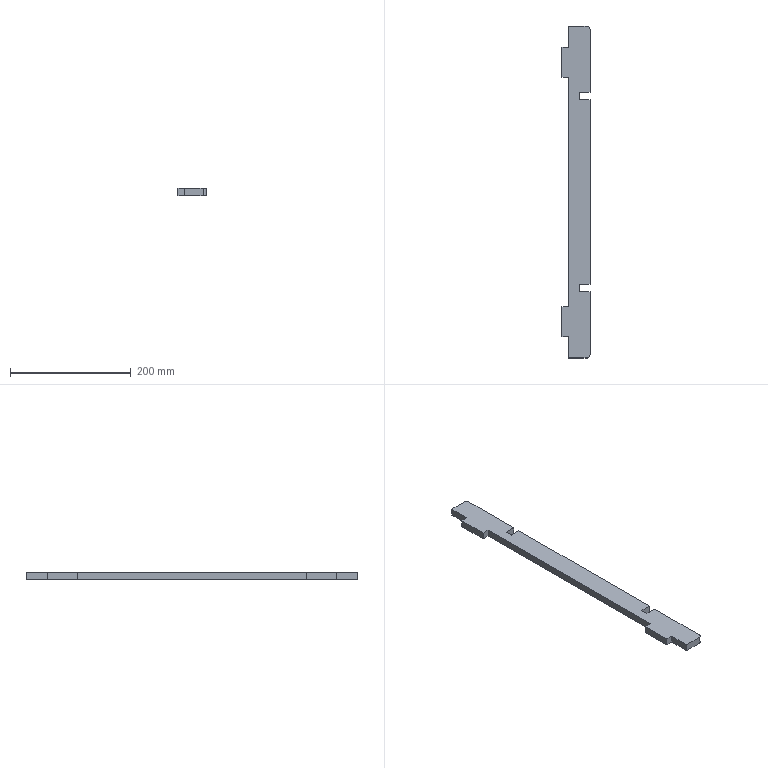Part | SolidWorks | features FlatPattern 1, SMBaseFlange 1, SheetMetal 1 | 1 solid | 24 faces | box 46.5 x 550 x 12 mm | volume 239574 mm3 | plane 22 | cylinder 2 | commonest cylinder face diameters 10 x2
STEP:
#1=CARTESIAN_POINT('',(-232.937,-290.509,0.));
#2=VERTEX_POINT('',#1);
#3=CARTESIAN_POINT('',(-232.937,-325.509,0.));
#4=VERTEX_POINT('',#3);
#5=CARTESIAN_POINT('',(-232.937,-325.509,0.));
#6=DIRECTION('',(0.,-1.,0.));
#7=VECTOR('',#6,1000.);
#8=LINE('',#5,#7);
#9=EDGE_CURVE('',#2,#4,#8,.T.);
#10=ORIENTED_EDGE('',*,*,#9,.F.);
#11=CARTESIAN_POINT('',(-232.937,-290.509,-12.));
#12=VERTEX_POINT('',#11);
#13=CARTESIAN_POINT('',(-232.937,-290.509,-12.));
#14=DIRECTION('',(0.,0.,1.));
#15=VECTOR('',#14,1000.);
#16=LINE('',#13,#15);
#17=EDGE_CURVE('',#12,#2,#16,.T.);
#18=ORIENTED_EDGE('',*,*,#17,.F.);
#19=CARTESIAN_POINT('',(-232.937,-325.509,-12.));
#20=VERTEX_POINT('',#19);
#21=CARTESIAN_POINT('',(-232.937,-325.509,-12.));
#22=DIRECTION('',(0.,-1.,0.));
#23=VECTOR('',#22,1000.);
#24=LINE('',#21,#23);
#25=EDGE_CURVE('',#12,#20,#24,.T.);
#26=ORIENTED_EDGE('',*,*,#25,.T.);
#27=CARTESIAN_POINT('',(-232.937,-325.509,-12.));
#28=DIRECTION('',(0.,0.,1.));
#29=VECTOR('',#28,1000.);
#30=LINE('',#27,#29);
#31=EDGE_CURVE('',#20,#4,#30,.T.);
#32=ORIENTED_EDGE('',*,*,#31,.T.);
#33=EDGE_LOOP('',(#10,#18,#26,#32));
#34=FACE_OUTER_BOUND('',#33,.T.);
#35=CARTESIAN_POINT('',(-232.937,-325.509,-12.));
#36=DIRECTION('',(-1.,0.,0.));
#37=DIRECTION('',(0.,0.,1.));
#38=AXIS2_PLACEMENT_3D('',#35,#36,#37);
#39=PLANE('',#38);
#40=ADVANCED_FACE('',(#34),#39,.T.);
#41=CARTESIAN_POINT('',(-244.437,-290.509,0.));
#42=VERTEX_POINT('',#41);
#43=CARTESIAN_POINT('',(-232.937,-290.509,0.));
#44=DIRECTION('',(1.,0.,0.));
#45=VECTOR('',#44,1000.);
#46=LINE('',#43,#45);
#47=EDGE_CURVE('',#42,#2,#46,.T.);
#48=ORIENTED_EDGE('',*,*,#47,.F.);
#49=CARTESIAN_POINT('',(-244.437,-290.509,-12.));
#50=VERTEX_POINT('',#49);
#51=CARTESIAN_POINT('',(-244.437,-290.509,-12.));
#52=DIRECTION('',(0.,0.,1.));
#53=VECTOR('',#52,1000.);
#54=LINE('',#51,#53);
#55=EDGE_CURVE('',#50,#42,#54,.T.);
#56=ORIENTED_EDGE('',*,*,#55,.F.);
#57=CARTESIAN_POINT('',(-232.937,-290.509,-12.));
#58=DIRECTION('',(1.,0.,0.));
#59=VECTOR('',#58,1000.);
#60=LINE('',#57,#59);
#61=EDGE_CURVE('',#50,#12,#60,.T.);
#62=ORIENTED_EDGE('',*,*,#61,.T.);
#63=ORIENTED_EDGE('',*,*,#17,.T.);
#64=EDGE_LOOP('',(#48,#56,#62,#63));
#65=FACE_OUTER_BOUND('',#64,.T.);
#66=CARTESIAN_POINT('',(-232.937,-290.509,-12.));
#67=DIRECTION('',(0.,-1.,0.));
#68=DIRECTION('',(0.,0.,-1.));
#69=AXIS2_PLACEMENT_3D('',#66,#67,#68);
#70=PLANE('',#69);
#71=ADVANCED_FACE('',(#65),#70,.T.);
#72=CARTESIAN_POINT('',(-244.437,-240.509,0.));
#73=VERTEX_POINT('',#72);
#74=CARTESIAN_POINT('',(-244.437,-290.509,0.));
#75=DIRECTION('',(0.,-1.,0.));
#76=VECTOR('',#75,1000.);
#77=LINE('',#74,#76);
#78=EDGE_CURVE('',#73,#42,#77,.T.);
#79=ORIENTED_EDGE('',*,*,#78,.F.);
#80=CARTESIAN_POINT('',(-244.437,-240.509,-12.));
#81=VERTEX_POINT('',#80);
#82=CARTESIAN_POINT('',(-244.437,-240.509,-12.));
#83=DIRECTION('',(0.,0.,1.));
#84=VECTOR('',#83,1000.);
#85=LINE('',#82,#84);
#86=EDGE_CURVE('',#81,#73,#85,.T.);
#87=ORIENTED_EDGE('',*,*,#86,.F.);
#88=CARTESIAN_POINT('',(-244.437,-290.509,-12.));
#89=DIRECTION('',(0.,-1.,0.));
#90=VECTOR('',#89,1000.);
#91=LINE('',#88,#90);
#92=EDGE_CURVE('',#81,#50,#91,.T.);
#93=ORIENTED_EDGE('',*,*,#92,.T.);
#94=ORIENTED_EDGE('',*,*,#55,.T.);
#95=EDGE_LOOP('',(#79,#87,#93,#94));
#96=FACE_OUTER_BOUND('',#95,.T.);
#97=CARTESIAN_POINT('',(-244.437,-290.509,-12.));
#98=DIRECTION('',(-1.,0.,0.));
#99=DIRECTION('',(0.,0.,1.));
#100=AXIS2_PLACEMENT_3D('',#97,#98,#99);
#101=PLANE('',#100);
#102=ADVANCED_FACE('',(#96),#101,.T.);
#103=CARTESIAN_POINT('',(-232.937,-240.509,0.));
#104=VERTEX_POINT('',#103);
#105=CARTESIAN_POINT('',(-244.437,-240.509,0.));
#106=DIRECTION('',(-1.,0.,0.));
#107=VECTOR('',#106,1000.);
#108=LINE('',#105,#107);
#109=EDGE_CURVE('',#104,#73,#108,.T.);
#110=ORIENTED_EDGE('',*,*,#109,.F.);
#111=CARTESIAN_POINT('',(-232.937,-240.509,-12.));
#112=VERTEX_POINT('',#111);
#113=CARTESIAN_POINT('',(-232.937,-240.509,-12.));
#114=DIRECTION('',(0.,0.,1.));
#115=VECTOR('',#114,1000.);
#116=LINE('',#113,#115);
#117=EDGE_CURVE('',#112,#104,#116,.T.);
#118=ORIENTED_EDGE('',*,*,#117,.F.);
#119=CARTESIAN_POINT('',(-244.437,-240.509,-12.));
#120=DIRECTION('',(-1.,0.,0.));
#121=VECTOR('',#120,1000.);
#122=LINE('',#119,#121);
#123=EDGE_CURVE('',#112,#81,#122,.T.);
#124=ORIENTED_EDGE('',*,*,#123,.T.);
#125=ORIENTED_EDGE('',*,*,#86,.T.);
#126=EDGE_LOOP('',(#110,#118,#124,#125));
#127=FACE_OUTER_BOUND('',#126,.T.);
#128=CARTESIAN_POINT('',(-244.437,-240.509,-12.));
#129=DIRECTION('',(0.,1.,0.));
#130=DIRECTION('',(-1.,0.,0.));
#131=AXIS2_PLACEMENT_3D('',#128,#129,#130);
#132=PLANE('',#131);
#133=ADVANCED_FACE('',(#127),#132,.T.);
#134=CARTESIAN_POINT('',(-232.937,139.491,0.));
#135=VERTEX_POINT('',#134);
#136=CARTESIAN_POINT('',(-232.937,-240.509,0.));
#137=DIRECTION('',(0.,-1.,0.));
#138=VECTOR('',#137,1000.);
#139=LINE('',#136,#138);
#140=EDGE_CURVE('',#135,#104,#139,.T.);
#141=ORIENTED_EDGE('',*,*,#140,.F.);
#142=CARTESIAN_POINT('',(-232.937,139.491,-12.));
#143=VERTEX_POINT('',#142);
#144=CARTESIAN_POINT('',(-232.937,139.491,-12.));
#145=DIRECTION('',(0.,0.,1.));
#146=VECTOR('',#145,1000.);
#147=LINE('',#144,#146);
#148=EDGE_CURVE('',#143,#135,#147,.T.);
#149=ORIENTED_EDGE('',*,*,#148,.F.);
#150=CARTESIAN_POINT('',(-232.937,-240.509,-12.));
#151=DIRECTION('',(0.,-1.,0.));
#152=VECTOR('',#151,1000.);
#153=LINE('',#150,#152);
#154=EDGE_CURVE('',#143,#112,#153,.T.);
#155=ORIENTED_EDGE('',*,*,#154,.T.);
#156=ORIENTED_EDGE('',*,*,#117,.T.);
#157=EDGE_LOOP('',(#141,#149,#155,#156));
#158=FACE_OUTER_BOUND('',#157,.T.);
#159=CARTESIAN_POINT('',(-232.937,-240.509,-12.));
#160=DIRECTION('',(-1.,0.,0.));
#161=DIRECTION('',(0.,0.,1.));
#162=AXIS2_PLACEMENT_3D('',#159,#160,#161);
#163=PLANE('',#162);
#164=ADVANCED_FACE('',(#158),#163,.T.);
#165=CARTESIAN_POINT('',(-244.437,139.491,0.));
#166=VERTEX_POINT('',#165);
#167=CARTESIAN_POINT('',(-244.437,139.491,0.));
#168=DIRECTION('',(1.,0.,0.));
#169=VECTOR('',#168,1000.);
#170=LINE('',#167,#169);
#171=EDGE_CURVE('',#166,#135,#170,.T.);
#172=ORIENTED_EDGE('',*,*,#171,.F.);
#173=CARTESIAN_POINT('',(-244.437,139.491,-12.));
#174=VERTEX_POINT('',#173);
#175=CARTESIAN_POINT('',(-244.437,139.491,-12.));
#176=DIRECTION('',(0.,0.,1.));
#177=VECTOR('',#176,1000.);
#178=LINE('',#175,#177);
#179=EDGE_CURVE('',#174,#166,#178,.T.);
#180=ORIENTED_EDGE('',*,*,#179,.F.);
#181=CARTESIAN_POINT('',(-244.437,139.491,-12.));
#182=DIRECTION('',(1.,0.,0.));
#183=VECTOR('',#182,1000.);
#184=LINE('',#181,#183);
#185=EDGE_CURVE('',#174,#143,#184,.T.);
#186=ORIENTED_EDGE('',*,*,#185,.T.);
#187=ORIENTED_EDGE('',*,*,#148,.T.);
#188=EDGE_LOOP('',(#172,#180,#186,#187));
#189=FACE_OUTER_BOUND('',#188,.T.);
#190=CARTESIAN_POINT('',(-244.437,139.491,-12.));
#191=DIRECTION('',(0.,-1.,0.));
#192=DIRECTION('',(0.,0.,-1.));
#193=AXIS2_PLACEMENT_3D('',#190,#191,#192);
#194=PLANE('',#193);
#195=ADVANCED_FACE('',(#189),#194,.T.);
#196=CARTESIAN_POINT('',(-244.437,189.491,0.));
#197=VERTEX_POINT('',#196);
#198=CARTESIAN_POINT('',(-244.437,189.491,0.));
#199=DIRECTION('',(0.,-1.,0.));
#200=VECTOR('',#199,1000.);
#201=LINE('',#198,#200);
#202=EDGE_CURVE('',#197,#166,#201,.T.);
#203=ORIENTED_EDGE('',*,*,#202,.F.);
#204=CARTESIAN_POINT('',(-244.437,189.491,-12.));
#205=VERTEX_POINT('',#204);
#206=CARTESIAN_POINT('',(-244.437,189.491,-12.));
#207=DIRECTION('',(0.,0.,1.));
#208=VECTOR('',#207,1000.);
#209=LINE('',#206,#208);
#210=EDGE_CURVE('',#205,#197,#209,.T.);
#211=ORIENTED_EDGE('',*,*,#210,.F.);
#212=CARTESIAN_POINT('',(-244.437,189.491,-12.));
#213=DIRECTION('',(0.,-1.,0.));
#214=VECTOR('',#213,1000.);
#215=LINE('',#212,#214);
#216=EDGE_CURVE('',#205,#174,#215,.T.);
#217=ORIENTED_EDGE('',*,*,#216,.T.);
#218=ORIENTED_EDGE('',*,*,#179,.T.);
#219=EDGE_LOOP('',(#203,#211,#217,#218));
#220=FACE_OUTER_BOUND('',#219,.T.);
#221=CARTESIAN_POINT('',(-244.437,189.491,-12.));
#222=DIRECTION('',(-1.,0.,0.));
#223=DIRECTION('',(0.,-1.,0.));
#224=AXIS2_PLACEMENT_3D('',#221,#222,#223);
#225=PLANE('',#224);
#226=ADVANCED_FACE('',(#220),#225,.T.);
#227=CARTESIAN_POINT('',(-232.937,189.491,0.));
#228=VERTEX_POINT('',#227);
#229=CARTESIAN_POINT('',(-232.937,189.491,0.));
#230=DIRECTION('',(-1.,0.,0.));
#231=VECTOR('',#230,1000.);
#232=LINE('',#229,#231);
#233=EDGE_CURVE('',#228,#197,#232,.T.);
#234=ORIENTED_EDGE('',*,*,#233,.F.);
#235=CARTESIAN_POINT('',(-232.937,189.491,-12.));
#236=VERTEX_POINT('',#235);
#237=CARTESIAN_POINT('',(-232.937,189.491,-12.));
#238=DIRECTION('',(0.,0.,1.));
#239=VECTOR('',#238,1000.);
#240=LINE('',#237,#239);
#241=EDGE_CURVE('',#236,#228,#240,.T.);
#242=ORIENTED_EDGE('',*,*,#241,.F.);
#243=CARTESIAN_POINT('',(-232.937,189.491,-12.));
#244=DIRECTION('',(-1.,0.,0.));
#245=VECTOR('',#244,1000.);
#246=LINE('',#243,#245);
#247=EDGE_CURVE('',#236,#205,#246,.T.);
#248=ORIENTED_EDGE('',*,*,#247,.T.);
#249=ORIENTED_EDGE('',*,*,#210,.T.);
#250=EDGE_LOOP('',(#234,#242,#248,#249));
#251=FACE_OUTER_BOUND('',#250,.T.);
#252=CARTESIAN_POINT('',(-232.937,189.491,-12.));
#253=DIRECTION('',(0.,1.,0.));
#254=DIRECTION('',(0.,0.,1.));
#255=AXIS2_PLACEMENT_3D('',#252,#253,#254);
#256=PLANE('',#255);
#257=ADVANCED_FACE('',(#251),#256,.T.);
#258=CARTESIAN_POINT('',(-232.937,224.491,0.));
#259=VERTEX_POINT('',#258);
#260=CARTESIAN_POINT('',(-232.937,189.491,0.));
#261=DIRECTION('',(0.,-1.,0.));
#262=VECTOR('',#261,1000.);
#263=LINE('',#260,#262);
#264=EDGE_CURVE('',#259,#228,#263,.T.);
#265=ORIENTED_EDGE('',*,*,#264,.F.);
#266=CARTESIAN_POINT('',(-232.937,224.491,-12.));
#267=VERTEX_POINT('',#266);
#268=CARTESIAN_POINT('',(-232.937,224.491,-12.));
#269=DIRECTION('',(0.,0.,1.));
#270=VECTOR('',#269,1000.);
#271=LINE('',#268,#270);
#272=EDGE_CURVE('',#267,#259,#271,.T.);
#273=ORIENTED_EDGE('',*,*,#272,.F.);
#274=CARTESIAN_POINT('',(-232.937,189.491,-12.));
#275=DIRECTION('',(0.,-1.,0.));
#276=VECTOR('',#275,1000.);
#277=LINE('',#274,#276);
#278=EDGE_CURVE('',#267,#236,#277,.T.);
#279=ORIENTED_EDGE('',*,*,#278,.T.);
#280=ORIENTED_EDGE('',*,*,#241,.T.);
#281=EDGE_LOOP('',(#265,#273,#279,#280));
#282=FACE_OUTER_BOUND('',#281,.T.);
#283=CARTESIAN_POINT('',(-232.937,189.491,-12.));
#284=DIRECTION('',(-1.,0.,0.));
#285=DIRECTION('',(0.,0.,1.));
#286=AXIS2_PLACEMENT_3D('',#283,#284,#285);
#287=PLANE('',#286);
#288=ADVANCED_FACE('',(#282),#287,.T.);
#289=CARTESIAN_POINT('',(-202.937,224.491,0.));
#290=VERTEX_POINT('',#289);
#291=CARTESIAN_POINT('',(-232.937,224.491,0.));
#292=DIRECTION('',(-1.,0.,0.));
#293=VECTOR('',#292,1000.);
#294=LINE('',#291,#293);
#295=EDGE_CURVE('',#290,#259,#294,.T.);
#296=ORIENTED_EDGE('',*,*,#295,.F.);
#297=CARTESIAN_POINT('',(-202.937,224.491,-12.));
#298=VERTEX_POINT('',#297);
#299=CARTESIAN_POINT('',(-202.937,224.491,-12.));
#300=DIRECTION('',(0.,0.,1.));
#301=VECTOR('',#300,1000.);
#302=LINE('',#299,#301);
#303=EDGE_CURVE('',#298,#290,#302,.T.);
#304=ORIENTED_EDGE('',*,*,#303,.F.);
#305=CARTESIAN_POINT('',(-232.937,224.491,-12.));
#306=DIRECTION('',(-1.,0.,0.));
#307=VECTOR('',#306,1000.);
#308=LINE('',#305,#307);
#309=EDGE_CURVE('',#298,#267,#308,.T.);
#310=ORIENTED_EDGE('',*,*,#309,.T.);
#311=ORIENTED_EDGE('',*,*,#272,.T.);
#312=EDGE_LOOP('',(#296,#304,#310,#311));
#313=FACE_OUTER_BOUND('',#312,.T.);
#314=CARTESIAN_POINT('',(-232.937,224.491,-12.));
#315=DIRECTION('',(0.,1.,0.));
#316=DIRECTION('',(0.,0.,1.));
#317=AXIS2_PLACEMENT_3D('',#314,#315,#316);
#318=PLANE('',#317);
#319=ADVANCED_FACE('',(#313),#318,.T.);
#320=CARTESIAN_POINT('',(-197.937,219.491,0.));
#321=VERTEX_POINT('',#320);
#322=CARTESIAN_POINT('',(-202.937,219.491,0.));
#323=DIRECTION('',(0.,0.,1.));
#324=DIRECTION('',(-1.,0.,0.));
#325=AXIS2_PLACEMENT_3D('',#322,#323,#324);
#326=CIRCLE('',#325,5.);
#327=EDGE_CURVE('',#321,#290,#326,.T.);
#328=ORIENTED_EDGE('',*,*,#327,.F.);
#329=CARTESIAN_POINT('',(-197.937,219.491,-12.));
#330=VERTEX_POINT('',#329);
#331=CARTESIAN_POINT('',(-197.937,219.491,-12.));
#332=DIRECTION('',(0.,0.,1.));
#333=VECTOR('',#332,1000.);
#334=LINE('',#331,#333);
#335=EDGE_CURVE('',#330,#321,#334,.T.);
#336=ORIENTED_EDGE('',*,*,#335,.F.);
#337=CARTESIAN_POINT('',(-202.937,219.491,-12.));
#338=DIRECTION('',(0.,0.,1.));
#339=DIRECTION('',(-1.,0.,0.));
#340=AXIS2_PLACEMENT_3D('',#337,#338,#339);
#341=CIRCLE('',#340,5.);
#342=EDGE_CURVE('',#330,#298,#341,.T.);
#343=ORIENTED_EDGE('',*,*,#342,.T.);
#344=ORIENTED_EDGE('',*,*,#303,.T.);
#345=EDGE_LOOP('',(#328,#336,#343,#344));
#346=FACE_OUTER_BOUND('',#345,.T.);
#347=CARTESIAN_POINT('',(-202.937,219.491,-12.));
#348=DIRECTION('',(0.,0.,1.));
#349=DIRECTION('',(1.,0.,0.));
#350=AXIS2_PLACEMENT_3D('',#347,#348,#349);
#351=CYLINDRICAL_SURFACE('',#350,5.);
#352=ADVANCED_FACE('',(#346),#351,.T.);
#353=CARTESIAN_POINT('',(-197.937,114.491,0.));
#354=VERTEX_POINT('',#353);
#355=CARTESIAN_POINT('',(-197.937,114.491,0.));
#356=DIRECTION('',(0.,1.,0.));
#357=VECTOR('',#356,1000.);
#358=LINE('',#355,#357);
#359=EDGE_CURVE('',#354,#321,#358,.T.);
#360=ORIENTED_EDGE('',*,*,#359,.F.);
#361=CARTESIAN_POINT('',(-197.937,114.491,-12.));
#362=VERTEX_POINT('',#361);
#363=CARTESIAN_POINT('',(-197.937,114.491,-12.));
#364=DIRECTION('',(0.,0.,1.));
#365=VECTOR('',#364,1000.);
#366=LINE('',#363,#365);
#367=EDGE_CURVE('',#362,#354,#366,.T.);
#368=ORIENTED_EDGE('',*,*,#367,.F.);
#369=CARTESIAN_POINT('',(-197.937,114.491,-12.));
#370=DIRECTION('',(0.,1.,0.));
#371=VECTOR('',#370,1000.);
#372=LINE('',#369,#371);
#373=EDGE_CURVE('',#362,#330,#372,.T.);
#374=ORIENTED_EDGE('',*,*,#373,.T.);
#375=ORIENTED_EDGE('',*,*,#335,.T.);
#376=EDGE_LOOP('',(#360,#368,#374,#375));
#377=FACE_OUTER_BOUND('',#376,.T.);
#378=CARTESIAN_POINT('',(-197.937,114.491,-12.));
#379=DIRECTION('',(1.,0.,0.));
#380=DIRECTION('',(0.,1.,0.));
#381=AXIS2_PLACEMENT_3D('',#378,#379,#380);
#382=PLANE('',#381);
#383=ADVANCED_FACE('',(#377),#382,.T.);
#384=CARTESIAN_POINT('',(-215.637,114.491,0.));
#385=VERTEX_POINT('',#384);
#386=CARTESIAN_POINT('',(-215.637,114.491,0.));
#387=DIRECTION('',(1.,0.,0.));
#388=VECTOR('',#387,1000.);
#389=LINE('',#386,#388);
#390=EDGE_CURVE('',#385,#354,#389,.T.);
#391=ORIENTED_EDGE('',*,*,#390,.F.);
#392=CARTESIAN_POINT('',(-215.637,114.491,-12.));
#393=VERTEX_POINT('',#392);
#394=CARTESIAN_POINT('',(-215.637,114.491,-12.));
#395=DIRECTION('',(0.,0.,1.));
#396=VECTOR('',#395,1000.);
#397=LINE('',#394,#396);
#398=EDGE_CURVE('',#393,#385,#397,.T.);
#399=ORIENTED_EDGE('',*,*,#398,.F.);
#400=CARTESIAN_POINT('',(-215.637,114.491,-12.));
#401=DIRECTION('',(1.,0.,0.));
#402=VECTOR('',#401,1000.);
#403=LINE('',#400,#402);
#404=EDGE_CURVE('',#393,#362,#403,.T.);
#405=ORIENTED_EDGE('',*,*,#404,.T.);
#406=ORIENTED_EDGE('',*,*,#367,.T.);
#407=EDGE_LOOP('',(#391,#399,#405,#406));
#408=FACE_OUTER_BOUND('',#407,.T.);
#409=CARTESIAN_POINT('',(-215.637,114.491,-12.));
#410=DIRECTION('',(0.,-1.,0.));
#411=DIRECTION('',(1.,0.,0.));
#412=AXIS2_PLACEMENT_3D('',#409,#410,#411);
#413=PLANE('',#412);
#414=ADVANCED_FACE('',(#408),#413,.T.);
#415=CARTESIAN_POINT('',(-215.637,102.491,0.));
#416=VERTEX_POINT('',#415);
#417=CARTESIAN_POINT('',(-215.637,102.491,0.));
#418=DIRECTION('',(0.,1.,0.));
#419=VECTOR('',#418,1000.);
#420=LINE('',#417,#419);
#421=EDGE_CURVE('',#416,#385,#420,.T.);
#422=ORIENTED_EDGE('',*,*,#421,.F.);
#423=CARTESIAN_POINT('',(-215.637,102.491,-12.));
#424=VERTEX_POINT('',#423);
#425=CARTESIAN_POINT('',(-215.637,102.491,-12.));
#426=DIRECTION('',(0.,0.,1.));
#427=VECTOR('',#426,1000.);
#428=LINE('',#425,#427);
#429=EDGE_CURVE('',#424,#416,#428,.T.);
#430=ORIENTED_EDGE('',*,*,#429,.F.);
#431=CARTESIAN_POINT('',(-215.637,102.491,-12.));
#432=DIRECTION('',(0.,1.,0.));
#433=VECTOR('',#432,1000.);
#434=LINE('',#431,#433);
#435=EDGE_CURVE('',#424,#393,#434,.T.);
#436=ORIENTED_EDGE('',*,*,#435,.T.);
#437=ORIENTED_EDGE('',*,*,#398,.T.);
#438=EDGE_LOOP('',(#422,#430,#436,#437));
#439=FACE_OUTER_BOUND('',#438,.T.);
#440=CARTESIAN_POINT('',(-215.637,102.491,-12.));
#441=DIRECTION('',(1.,0.,0.));
#442=DIRECTION('',(0.,0.,-1.));
#443=AXIS2_PLACEMENT_3D('',#440,#441,#442);
#444=PLANE('',#443);
#445=ADVANCED_FACE('',(#439),#444,.T.);
#446=CARTESIAN_POINT('',(-197.937,102.491,0.));
#447=VERTEX_POINT('',#446);
#448=CARTESIAN_POINT('',(-197.937,102.491,0.));
#449=DIRECTION('',(-1.,0.,0.));
#450=VECTOR('',#449,1000.);
#451=LINE('',#448,#450);
#452=EDGE_CURVE('',#447,#416,#451,.T.);
#453=ORIENTED_EDGE('',*,*,#452,.F.);
#454=CARTESIAN_POINT('',(-197.937,102.491,-12.));
#455=VERTEX_POINT('',#454);
#456=CARTESIAN_POINT('',(-197.937,102.491,-12.));
#457=DIRECTION('',(0.,0.,1.));
#458=VECTOR('',#457,1000.);
#459=LINE('',#456,#458);
#460=EDGE_CURVE('',#455,#447,#459,.T.);
#461=ORIENTED_EDGE('',*,*,#460,.F.);
#462=CARTESIAN_POINT('',(-197.937,102.491,-12.));
#463=DIRECTION('',(-1.,0.,0.));
#464=VECTOR('',#463,1000.);
#465=LINE('',#462,#464);
#466=EDGE_CURVE('',#455,#424,#465,.T.);
#467=ORIENTED_EDGE('',*,*,#466,.T.);
#468=ORIENTED_EDGE('',*,*,#429,.T.);
#469=EDGE_LOOP('',(#453,#461,#467,#468));
#470=FACE_OUTER_BOUND('',#469,.T.);
#471=CARTESIAN_POINT('',(-197.937,102.491,-12.));
#472=DIRECTION('',(0.,1.,0.));
#473=DIRECTION('',(-1.,0.,0.));
#474=AXIS2_PLACEMENT_3D('',#471,#472,#473);
#475=PLANE('',#474);
#476=ADVANCED_FACE('',(#470),#475,.T.);
#477=CARTESIAN_POINT('',(-197.937,-203.509,0.));
#478=VERTEX_POINT('',#477);
#479=CARTESIAN_POINT('',(-197.937,-203.509,0.));
#480=DIRECTION('',(0.,1.,0.));
#481=VECTOR('',#480,1000.);
#482=LINE('',#479,#481);
#483=EDGE_CURVE('',#478,#447,#482,.T.);
#484=ORIENTED_EDGE('',*,*,#483,.F.);
#485=CARTESIAN_POINT('',(-197.937,-203.509,-12.));
#486=VERTEX_POINT('',#485);
#487=CARTESIAN_POINT('',(-197.937,-203.509,-12.));
#488=DIRECTION('',(0.,0.,1.));
#489=VECTOR('',#488,1000.);
#490=LINE('',#487,#489);
#491=EDGE_CURVE('',#486,#478,#490,.T.);
#492=ORIENTED_EDGE('',*,*,#491,.F.);
#493=CARTESIAN_POINT('',(-197.937,-203.509,-12.));
#494=DIRECTION('',(0.,1.,0.));
#495=VECTOR('',#494,1000.);
#496=LINE('',#493,#495);
#497=EDGE_CURVE('',#486,#455,#496,.T.);
#498=ORIENTED_EDGE('',*,*,#497,.T.);
#499=ORIENTED_EDGE('',*,*,#460,.T.);
#500=EDGE_LOOP('',(#484,#492,#498,#499));
#501=FACE_OUTER_BOUND('',#500,.T.);
#502=CARTESIAN_POINT('',(-197.937,-203.509,-12.));
#503=DIRECTION('',(1.,0.,0.));
#504=DIRECTION('',(0.,1.,0.));
#505=AXIS2_PLACEMENT_3D('',#502,#503,#504);
#506=PLANE('',#505);
#507=ADVANCED_FACE('',(#501),#506,.T.);
#508=CARTESIAN_POINT('',(-215.637,-203.509,0.));
#509=VERTEX_POINT('',#508);
#510=CARTESIAN_POINT('',(-215.637,-203.509,0.));
#511=DIRECTION('',(1.,0.,0.));
#512=VECTOR('',#511,1000.);
#513=LINE('',#510,#512);
#514=EDGE_CURVE('',#509,#478,#513,.T.);
#515=ORIENTED_EDGE('',*,*,#514,.F.);
#516=CARTESIAN_POINT('',(-215.637,-203.509,-12.));
#517=VERTEX_POINT('',#516);
#518=CARTESIAN_POINT('',(-215.637,-203.509,-12.));
#519=DIRECTION('',(0.,0.,1.));
#520=VECTOR('',#519,1000.);
#521=LINE('',#518,#520);
#522=EDGE_CURVE('',#517,#509,#521,.T.);
#523=ORIENTED_EDGE('',*,*,#522,.F.);
#524=CARTESIAN_POINT('',(-215.637,-203.509,-12.));
#525=DIRECTION('',(1.,0.,0.));
#526=VECTOR('',#525,1000.);
#527=LINE('',#524,#526);
#528=EDGE_CURVE('',#517,#486,#527,.T.);
#529=ORIENTED_EDGE('',*,*,#528,.T.);
#530=ORIENTED_EDGE('',*,*,#491,.T.);
#531=EDGE_LOOP('',(#515,#523,#529,#530));
#532=FACE_OUTER_BOUND('',#531,.T.);
#533=CARTESIAN_POINT('',(-215.637,-203.509,-12.));
#534=DIRECTION('',(0.,-1.,0.));
#535=DIRECTION('',(0.,0.,-1.));
#536=AXIS2_PLACEMENT_3D('',#533,#534,#535);
#537=PLANE('',#536);
#538=ADVANCED_FACE('',(#532),#537,.T.);
#539=CARTESIAN_POINT('',(-215.637,-215.509,0.));
#540=VERTEX_POINT('',#539);
#541=CARTESIAN_POINT('',(-215.637,-215.509,0.));
#542=DIRECTION('',(0.,1.,0.));
#543=VECTOR('',#542,1000.);
#544=LINE('',#541,#543);
#545=EDGE_CURVE('',#540,#509,#544,.T.);
#546=ORIENTED_EDGE('',*,*,#545,.F.);
#547=CARTESIAN_POINT('',(-215.637,-215.509,-12.));
#548=VERTEX_POINT('',#547);
#549=CARTESIAN_POINT('',(-215.637,-215.509,-12.));
#550=DIRECTION('',(0.,0.,1.));
#551=VECTOR('',#550,1000.);
#552=LINE('',#549,#551);
#553=EDGE_CURVE('',#548,#540,#552,.T.);
#554=ORIENTED_EDGE('',*,*,#553,.F.);
#555=CARTESIAN_POINT('',(-215.637,-215.509,-12.));
#556=DIRECTION('',(0.,1.,0.));
#557=VECTOR('',#556,1000.);
#558=LINE('',#555,#557);
#559=EDGE_CURVE('',#548,#517,#558,.T.);
#560=ORIENTED_EDGE('',*,*,#559,.T.);
#561=ORIENTED_EDGE('',*,*,#522,.T.);
#562=EDGE_LOOP('',(#546,#554,#560,#561));
#563=FACE_OUTER_BOUND('',#562,.T.);
#564=CARTESIAN_POINT('',(-215.637,-215.509,-12.));
#565=DIRECTION('',(1.,0.,0.));
#566=DIRECTION('',(0.,1.,0.));
#567=AXIS2_PLACEMENT_3D('',#564,#565,#566);
#568=PLANE('',#567);
#569=ADVANCED_FACE('',(#563),#568,.T.);
#570=CARTESIAN_POINT('',(-197.937,-215.509,0.));
#571=VERTEX_POINT('',#570);
#572=CARTESIAN_POINT('',(-197.937,-215.509,0.));
#573=DIRECTION('',(-1.,0.,0.));
#574=VECTOR('',#573,1000.);
#575=LINE('',#572,#574);
#576=EDGE_CURVE('',#571,#540,#575,.T.);
#577=ORIENTED_EDGE('',*,*,#576,.F.);
#578=CARTESIAN_POINT('',(-197.937,-215.509,-12.));
#579=VERTEX_POINT('',#578);
#580=CARTESIAN_POINT('',(-197.937,-215.509,-12.));
#581=DIRECTION('',(0.,0.,1.));
#582=VECTOR('',#581,1000.);
#583=LINE('',#580,#582);
#584=EDGE_CURVE('',#579,#571,#583,.T.);
#585=ORIENTED_EDGE('',*,*,#584,.F.);
#586=CARTESIAN_POINT('',(-197.937,-215.509,-12.));
#587=DIRECTION('',(-1.,0.,0.));
#588=VECTOR('',#587,1000.);
#589=LINE('',#586,#588);
#590=EDGE_CURVE('',#579,#548,#589,.T.);
#591=ORIENTED_EDGE('',*,*,#590,.T.);
#592=ORIENTED_EDGE('',*,*,#553,.T.);
#593=EDGE_LOOP('',(#577,#585,#591,#592));
#594=FACE_OUTER_BOUND('',#593,.T.);
#595=CARTESIAN_POINT('',(-197.937,-215.509,-12.));
#596=DIRECTION('',(0.,1.,0.));
#597=DIRECTION('',(0.,0.,1.));
#598=AXIS2_PLACEMENT_3D('',#595,#596,#597);
#599=PLANE('',#598);
#600=ADVANCED_FACE('',(#594),#599,.T.);
#601=CARTESIAN_POINT('',(-197.937,-320.509,0.));
#602=VERTEX_POINT('',#601);
#603=CARTESIAN_POINT('',(-197.937,-320.509,0.));
#604=DIRECTION('',(0.,1.,0.));
#605=VECTOR('',#604,1000.);
#606=LINE('',#603,#605);
#607=EDGE_CURVE('',#602,#571,#606,.T.);
#608=ORIENTED_EDGE('',*,*,#607,.F.);
#609=CARTESIAN_POINT('',(-197.937,-320.509,-12.));
#610=VERTEX_POINT('',#609);
#611=CARTESIAN_POINT('',(-197.937,-320.509,-12.));
#612=DIRECTION('',(0.,0.,1.));
#613=VECTOR('',#612,1000.);
#614=LINE('',#611,#613);
#615=EDGE_CURVE('',#610,#602,#614,.T.);
#616=ORIENTED_EDGE('',*,*,#615,.F.);
#617=CARTESIAN_POINT('',(-197.937,-320.509,-12.));
#618=DIRECTION('',(0.,1.,0.));
#619=VECTOR('',#618,1000.);
#620=LINE('',#617,#619);
#621=EDGE_CURVE('',#610,#579,#620,.T.);
#622=ORIENTED_EDGE('',*,*,#621,.T.);
#623=ORIENTED_EDGE('',*,*,#584,.T.);
#624=EDGE_LOOP('',(#608,#616,#622,#623));
#625=FACE_OUTER_BOUND('',#624,.T.);
#626=CARTESIAN_POINT('',(-197.937,-320.509,-12.));
#627=DIRECTION('',(1.,0.,0.));
#628=DIRECTION('',(0.,0.,-1.));
#629=AXIS2_PLACEMENT_3D('',#626,#627,#628);
#630=PLANE('',#629);
#631=ADVANCED_FACE('',(#625),#630,.T.);
#632=CARTESIAN_POINT('',(-202.937,-325.509,0.));
#633=VERTEX_POINT('',#632);
#634=CARTESIAN_POINT('',(-202.937,-320.509,0.));
#635=DIRECTION('',(0.,0.,1.));
#636=DIRECTION('',(1.,0.,0.));
#637=AXIS2_PLACEMENT_3D('',#634,#635,#636);
#638=CIRCLE('',#637,5.);
#639=EDGE_CURVE('',#633,#602,#638,.T.);
#640=ORIENTED_EDGE('',*,*,#639,.F.);
#641=CARTESIAN_POINT('',(-202.937,-325.509,-12.));
#642=VERTEX_POINT('',#641);
#643=CARTESIAN_POINT('',(-202.937,-325.509,-12.));
#644=DIRECTION('',(0.,0.,1.));
#645=VECTOR('',#644,1000.);
#646=LINE('',#643,#645);
#647=EDGE_CURVE('',#642,#633,#646,.T.);
#648=ORIENTED_EDGE('',*,*,#647,.F.);
#649=CARTESIAN_POINT('',(-202.937,-320.509,-12.));
#650=DIRECTION('',(0.,0.,1.));
#651=DIRECTION('',(1.,0.,0.));
#652=AXIS2_PLACEMENT_3D('',#649,#650,#651);
#653=CIRCLE('',#652,5.);
#654=EDGE_CURVE('',#642,#610,#653,.T.);
#655=ORIENTED_EDGE('',*,*,#654,.T.);
#656=ORIENTED_EDGE('',*,*,#615,.T.);
#657=EDGE_LOOP('',(#640,#648,#655,#656));
#658=FACE_OUTER_BOUND('',#657,.T.);
#659=CARTESIAN_POINT('',(-202.937,-320.509,-12.));
#660=DIRECTION('',(0.,0.,1.));
#661=DIRECTION('',(1.,0.,0.));
#662=AXIS2_PLACEMENT_3D('',#659,#660,#661);
#663=CYLINDRICAL_SURFACE('',#662,5.);
#664=ADVANCED_FACE('',(#658),#663,.T.);
#665=CARTESIAN_POINT('',(-232.937,-325.509,0.));
#666=DIRECTION('',(1.,0.,0.));
#667=VECTOR('',#666,1000.);
#668=LINE('',#665,#667);
#669=EDGE_CURVE('',#4,#633,#668,.T.);
#670=ORIENTED_EDGE('',*,*,#669,.F.);
#671=ORIENTED_EDGE('',*,*,#31,.F.);
#672=CARTESIAN_POINT('',(-232.937,-325.509,-12.));
#673=DIRECTION('',(1.,0.,0.));
#674=VECTOR('',#673,1000.);
#675=LINE('',#672,#674);
#676=EDGE_CURVE('',#20,#642,#675,.T.);
#677=ORIENTED_EDGE('',*,*,#676,.T.);
#678=ORIENTED_EDGE('',*,*,#647,.T.);
#679=EDGE_LOOP('',(#670,#671,#677,#678));
#680=FACE_OUTER_BOUND('',#679,.T.);
#681=CARTESIAN_POINT('',(-232.937,-325.509,-12.));
#682=DIRECTION('',(0.,-1.,0.));
#683=DIRECTION('',(0.,0.,-1.));
#684=AXIS2_PLACEMENT_3D('',#681,#682,#683);
#685=PLANE('',#684);
#686=ADVANCED_FACE('',(#680),#685,.T.);
#687=ORIENTED_EDGE('',*,*,#25,.F.);
#688=ORIENTED_EDGE('',*,*,#61,.F.);
#689=ORIENTED_EDGE('',*,*,#92,.F.);
#690=ORIENTED_EDGE('',*,*,#123,.F.);
#691=ORIENTED_EDGE('',*,*,#154,.F.);
#692=ORIENTED_EDGE('',*,*,#185,.F.);
#693=ORIENTED_EDGE('',*,*,#216,.F.);
#694=ORIENTED_EDGE('',*,*,#247,.F.);
#695=ORIENTED_EDGE('',*,*,#278,.F.);
#696=ORIENTED_EDGE('',*,*,#309,.F.);
#697=ORIENTED_EDGE('',*,*,#342,.F.);
#698=ORIENTED_EDGE('',*,*,#373,.F.);
#699=ORIENTED_EDGE('',*,*,#404,.F.);
#700=ORIENTED_EDGE('',*,*,#435,.F.);
#701=ORIENTED_EDGE('',*,*,#466,.F.);
#702=ORIENTED_EDGE('',*,*,#497,.F.);
#703=ORIENTED_EDGE('',*,*,#528,.F.);
#704=ORIENTED_EDGE('',*,*,#559,.F.);
#705=ORIENTED_EDGE('',*,*,#590,.F.);
#706=ORIENTED_EDGE('',*,*,#621,.F.);
#707=ORIENTED_EDGE('',*,*,#654,.F.);
#708=ORIENTED_EDGE('',*,*,#676,.F.);
#709=EDGE_LOOP('',(#687,#688,#689,#690,#691,#692,#693,#694,#695,#696,#697,#698,#699,#700,#701,#702,#703,#704,#705,#706,#707,#708));
#710=FACE_OUTER_BOUND('',#709,.T.);
#711=CARTESIAN_POINT('',(-202.937,219.491,-12.));
#712=DIRECTION('',(0.,0.,-1.));
#713=DIRECTION('',(-1.,0.,0.));
#714=AXIS2_PLACEMENT_3D('',#711,#712,#713);
#715=PLANE('',#714);
#716=ADVANCED_FACE('',(#710),#715,.T.);
#717=ORIENTED_EDGE('',*,*,#9,.T.);
#718=ORIENTED_EDGE('',*,*,#669,.T.);
#719=ORIENTED_EDGE('',*,*,#639,.T.);
#720=ORIENTED_EDGE('',*,*,#607,.T.);
#721=ORIENTED_EDGE('',*,*,#576,.T.);
#722=ORIENTED_EDGE('',*,*,#545,.T.);
#723=ORIENTED_EDGE('',*,*,#514,.T.);
#724=ORIENTED_EDGE('',*,*,#483,.T.);
#725=ORIENTED_EDGE('',*,*,#452,.T.);
#726=ORIENTED_EDGE('',*,*,#421,.T.);
#727=ORIENTED_EDGE('',*,*,#390,.T.);
#728=ORIENTED_EDGE('',*,*,#359,.T.);
#729=ORIENTED_EDGE('',*,*,#327,.T.);
#730=ORIENTED_EDGE('',*,*,#295,.T.);
#731=ORIENTED_EDGE('',*,*,#264,.T.);
#732=ORIENTED_EDGE('',*,*,#233,.T.);
#733=ORIENTED_EDGE('',*,*,#202,.T.);
#734=ORIENTED_EDGE('',*,*,#171,.T.);
#735=ORIENTED_EDGE('',*,*,#140,.T.);
#736=ORIENTED_EDGE('',*,*,#109,.T.);
#737=ORIENTED_EDGE('',*,*,#78,.T.);
#738=ORIENTED_EDGE('',*,*,#47,.T.);
#739=EDGE_LOOP('',(#717,#718,#719,#720,#721,#722,#723,#724,#725,#726,#727,#728,#729,#730,#731,#732,#733,#734,#735,#736,#737,#738));
#740=FACE_OUTER_BOUND('',#739,.T.);
#741=CARTESIAN_POINT('',(-202.937,219.491,0.));
#742=DIRECTION('',(0.,0.,-1.));
#743=DIRECTION('',(-1.,0.,0.));
#744=AXIS2_PLACEMENT_3D('',#741,#742,#743);
#745=PLANE('',#744);
#746=ADVANCED_FACE('',(#740),#745,.F.);
#747=CLOSED_SHELL('',(#40,#71,#102,#133,#164,#195,#226,#257,#288,#319,#352,#383,#414,#445,#476,#507,#538,#569,#600,#631,#664,#686,#716,#746));
#748=MANIFOLD_SOLID_BREP('',#747);
#749=CARTESIAN_POINT('',(0.,0.,0.));
#750=DIRECTION('',(0.,0.,1.));
#751=DIRECTION('',(1.,0.,0.));
#752=AXIS2_PLACEMENT_3D('',#749,#750,#751);
#753=(LENGTH_UNIT()NAMED_UNIT(*)SI_UNIT(.MILLI.,.METRE.));
#754=UNCERTAINTY_MEASURE_WITH_UNIT(LENGTH_MEASURE(0.00001),#753,'','');
#755=(NAMED_UNIT(*)PLANE_ANGLE_UNIT()SI_UNIT($,.RADIAN.));
#756=(NAMED_UNIT(*)SI_UNIT($,.STERADIAN.)SOLID_ANGLE_UNIT());
#757=(GEOMETRIC_REPRESENTATION_CONTEXT(3)GLOBAL_UNCERTAINTY_ASSIGNED_CONTEXT((#754))GLOBAL_UNIT_ASSIGNED_CONTEXT((#753,#755,#756))REPRESENTATION_CONTEXT('',''));
#758=ADVANCED_BREP_SHAPE_REPRESENTATION('',(#748,#752),#757);